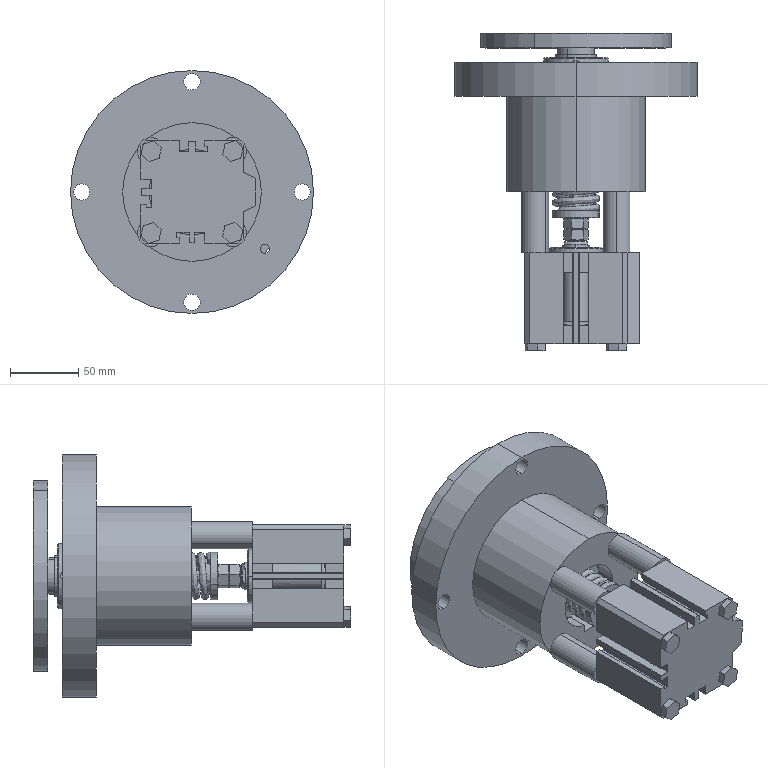Part | SolidWorks | 19 solids | 480 faces | box 178.5 x 233.2 x 178.5 mm | volume 1520245 mm3 | cylinder 201 | plane 190 | cone 75 | spline 14 | commonest cylinder face diameters 11 x52 8 x16 9 x16 20 x12 6.8 x10 12 x10